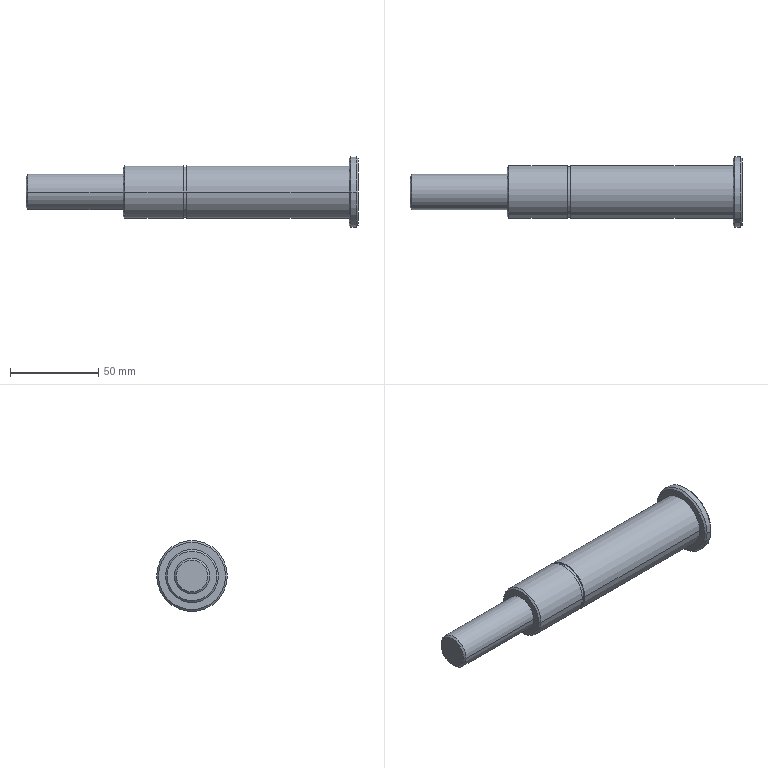Part | SolidWorks | features BaseBody 1 | 1 solid | 24 faces | box 188 x 40 x 40 mm | volume 113711 mm3 | cylinder 10 | cone 8 | plane 6 | commonest cylinder face diameters 30 x4 20 x2 28.6 x2 40 x2
STEP:
#1=CARTESIAN_POINT('',(89.,-19.,0.));
#2=VERTEX_POINT('',#1);
#3=CARTESIAN_POINT('',(89.,19.,0.));
#4=VERTEX_POINT('',#3);
#5=CARTESIAN_POINT('',(89.,0.,0.));
#6=DIRECTION('',(-1.,0.,0.));
#7=DIRECTION('',(0.,1.,0.));
#8=AXIS2_PLACEMENT_3D('',#5,#6,#7);
#9=CIRCLE('',#8,19.);
#10=EDGE_CURVE('',#2,#4,#9,.T.);
#11=ORIENTED_EDGE('',*,*,#10,.F.);
#12=CARTESIAN_POINT('',(90.,-20.,0.));
#13=VERTEX_POINT('',#12);
#14=CARTESIAN_POINT('',(89.,-19.,0.));
#15=DIRECTION('',(0.7071,-0.7071,0.));
#16=VECTOR('',#15,1000.);
#17=LINE('',#14,#16);
#18=EDGE_CURVE('',#2,#13,#17,.T.);
#19=ORIENTED_EDGE('',*,*,#18,.T.);
#20=CARTESIAN_POINT('',(90.,20.,0.));
#21=VERTEX_POINT('',#20);
#22=CARTESIAN_POINT('',(90.,0.,0.));
#23=DIRECTION('',(1.,0.,0.));
#24=DIRECTION('',(0.,1.,0.));
#25=AXIS2_PLACEMENT_3D('',#22,#23,#24);
#26=CIRCLE('',#25,20.);
#27=EDGE_CURVE('',#21,#13,#26,.T.);
#28=ORIENTED_EDGE('',*,*,#27,.F.);
#29=CARTESIAN_POINT('',(89.,19.,0.));
#30=DIRECTION('',(0.7071,0.7071,0.));
#31=VECTOR('',#30,1000.);
#32=LINE('',#29,#31);
#33=EDGE_CURVE('',#4,#21,#32,.T.);
#34=ORIENTED_EDGE('',*,*,#33,.F.);
#35=EDGE_LOOP('',(#11,#19,#28,#34));
#36=FACE_OUTER_BOUND('',#35,.T.);
#37=CARTESIAN_POINT('',(89.,0.,0.));
#38=DIRECTION('',(1.,0.,0.));
#39=DIRECTION('',(0.,1.,0.));
#40=AXIS2_PLACEMENT_3D('',#37,#38,#39);
#41=CONICAL_SURFACE('',#40,19.,0.7854);
#42=ADVANCED_FACE('',(#36),#41,.T.);
#43=CARTESIAN_POINT('',(94.,19.,0.));
#44=VERTEX_POINT('',#43);
#45=CARTESIAN_POINT('',(94.,-19.,0.));
#46=VERTEX_POINT('',#45);
#47=CARTESIAN_POINT('',(94.,0.,0.));
#48=DIRECTION('',(1.,0.,0.));
#49=DIRECTION('',(0.,-1.,0.));
#50=AXIS2_PLACEMENT_3D('',#47,#48,#49);
#51=CIRCLE('',#50,19.);
#52=EDGE_CURVE('',#44,#46,#51,.T.);
#53=ORIENTED_EDGE('',*,*,#52,.F.);
#54=CARTESIAN_POINT('',(93.,20.,0.));
#55=VERTEX_POINT('',#54);
#56=CARTESIAN_POINT('',(93.,20.,0.));
#57=DIRECTION('',(-0.7071,0.7071,0.));
#58=VECTOR('',#57,1000.);
#59=LINE('',#56,#58);
#60=EDGE_CURVE('',#44,#55,#59,.T.);
#61=ORIENTED_EDGE('',*,*,#60,.T.);
#62=CARTESIAN_POINT('',(93.,-20.,0.));
#63=VERTEX_POINT('',#62);
#64=CARTESIAN_POINT('',(93.,0.,0.));
#65=DIRECTION('',(-1.,0.,0.));
#66=DIRECTION('',(0.,-1.,0.));
#67=AXIS2_PLACEMENT_3D('',#64,#65,#66);
#68=CIRCLE('',#67,20.);
#69=EDGE_CURVE('',#63,#55,#68,.T.);
#70=ORIENTED_EDGE('',*,*,#69,.F.);
#71=CARTESIAN_POINT('',(93.,-20.,0.));
#72=DIRECTION('',(-0.7071,-0.7071,0.));
#73=VECTOR('',#72,1000.);
#74=LINE('',#71,#73);
#75=EDGE_CURVE('',#46,#63,#74,.T.);
#76=ORIENTED_EDGE('',*,*,#75,.F.);
#77=EDGE_LOOP('',(#53,#61,#70,#76));
#78=FACE_OUTER_BOUND('',#77,.T.);
#79=CARTESIAN_POINT('',(93.,0.,0.));
#80=DIRECTION('',(-1.,0.,0.));
#81=DIRECTION('',(0.,-1.,0.));
#82=AXIS2_PLACEMENT_3D('',#79,#80,#81);
#83=CONICAL_SURFACE('',#82,20.,0.7854);
#84=ADVANCED_FACE('',(#78),#83,.T.);
#85=CARTESIAN_POINT('',(-94.,-9.,0.));
#86=VERTEX_POINT('',#85);
#87=CARTESIAN_POINT('',(-94.,9.,0.));
#88=VERTEX_POINT('',#87);
#89=CARTESIAN_POINT('',(-94.,0.,0.));
#90=DIRECTION('',(-1.,0.,0.));
#91=DIRECTION('',(0.,-1.,0.));
#92=AXIS2_PLACEMENT_3D('',#89,#90,#91);
#93=CIRCLE('',#92,9.);
#94=EDGE_CURVE('',#86,#88,#93,.T.);
#95=ORIENTED_EDGE('',*,*,#94,.F.);
#96=CARTESIAN_POINT('',(-93.,-10.,0.));
#97=VERTEX_POINT('',#96);
#98=CARTESIAN_POINT('',(-93.,-10.,0.));
#99=DIRECTION('',(0.7071,-0.7071,0.));
#100=VECTOR('',#99,1000.);
#101=LINE('',#98,#100);
#102=EDGE_CURVE('',#86,#97,#101,.T.);
#103=ORIENTED_EDGE('',*,*,#102,.T.);
#104=CARTESIAN_POINT('',(-93.,10.,0.));
#105=VERTEX_POINT('',#104);
#106=CARTESIAN_POINT('',(-93.,0.,0.));
#107=DIRECTION('',(-1.,0.,0.));
#108=DIRECTION('',(0.,-1.,0.));
#109=AXIS2_PLACEMENT_3D('',#106,#107,#108);
#110=CIRCLE('',#109,10.);
#111=EDGE_CURVE('',#97,#105,#110,.T.);
#112=ORIENTED_EDGE('',*,*,#111,.T.);
#113=CARTESIAN_POINT('',(-93.,10.,0.));
#114=DIRECTION('',(0.7071,0.7071,0.));
#115=VECTOR('',#114,1000.);
#116=LINE('',#113,#115);
#117=EDGE_CURVE('',#88,#105,#116,.T.);
#118=ORIENTED_EDGE('',*,*,#117,.F.);
#119=EDGE_LOOP('',(#95,#103,#112,#118));
#120=FACE_OUTER_BOUND('',#119,.T.);
#121=CARTESIAN_POINT('',(-93.,0.,0.));
#122=DIRECTION('',(1.,0.,0.));
#123=DIRECTION('',(0.,1.,0.));
#124=AXIS2_PLACEMENT_3D('',#121,#122,#123);
#125=CONICAL_SURFACE('',#124,10.,0.7854);
#126=ADVANCED_FACE('',(#120),#125,.T.);
#127=CARTESIAN_POINT('',(-39.,-10.,0.));
#128=VERTEX_POINT('',#127);
#129=CARTESIAN_POINT('',(-39.,10.,0.));
#130=VERTEX_POINT('',#129);
#131=CARTESIAN_POINT('',(-39.,0.,0.));
#132=DIRECTION('',(-1.,0.,0.));
#133=DIRECTION('',(0.,-1.,0.));
#134=AXIS2_PLACEMENT_3D('',#131,#132,#133);
#135=CIRCLE('',#134,10.);
#136=EDGE_CURVE('',#128,#130,#135,.T.);
#137=ORIENTED_EDGE('',*,*,#136,.T.);
#138=CARTESIAN_POINT('',(-94.,10.,0.));
#139=DIRECTION('',(-1.,0.,0.));
#140=VECTOR('',#139,1000.);
#141=LINE('',#138,#140);
#142=EDGE_CURVE('',#130,#105,#141,.T.);
#143=ORIENTED_EDGE('',*,*,#142,.T.);
#144=ORIENTED_EDGE('',*,*,#111,.F.);
#145=CARTESIAN_POINT('',(-94.,-10.,0.));
#146=DIRECTION('',(-1.,0.,0.));
#147=VECTOR('',#146,1000.);
#148=LINE('',#145,#147);
#149=EDGE_CURVE('',#128,#97,#148,.T.);
#150=ORIENTED_EDGE('',*,*,#149,.F.);
#151=EDGE_LOOP('',(#137,#143,#144,#150));
#152=FACE_OUTER_BOUND('',#151,.T.);
#153=CARTESIAN_POINT('',(-94.,0.,0.));
#154=DIRECTION('',(-1.,0.,0.));
#155=DIRECTION('',(0.,-1.,0.));
#156=AXIS2_PLACEMENT_3D('',#153,#154,#155);
#157=CYLINDRICAL_SURFACE('',#156,10.);
#158=ADVANCED_FACE('',(#152),#157,.T.);
#159=CARTESIAN_POINT('',(-39.,-14.,0.));
#160=VERTEX_POINT('',#159);
#161=CARTESIAN_POINT('',(-39.,14.,0.));
#162=VERTEX_POINT('',#161);
#163=CARTESIAN_POINT('',(-39.,0.,0.));
#164=DIRECTION('',(-1.,0.,0.));
#165=DIRECTION('',(0.,-1.,0.));
#166=AXIS2_PLACEMENT_3D('',#163,#164,#165);
#167=CIRCLE('',#166,14.);
#168=EDGE_CURVE('',#160,#162,#167,.T.);
#169=ORIENTED_EDGE('',*,*,#168,.F.);
#170=CARTESIAN_POINT('',(-38.,-15.,0.));
#171=VERTEX_POINT('',#170);
#172=CARTESIAN_POINT('',(-38.,-15.,0.));
#173=DIRECTION('',(0.7071,-0.7071,0.));
#174=VECTOR('',#173,1000.);
#175=LINE('',#172,#174);
#176=EDGE_CURVE('',#160,#171,#175,.T.);
#177=ORIENTED_EDGE('',*,*,#176,.T.);
#178=CARTESIAN_POINT('',(-38.,15.,0.));
#179=VERTEX_POINT('',#178);
#180=CARTESIAN_POINT('',(-38.,0.,0.));
#181=DIRECTION('',(-1.,0.,0.));
#182=DIRECTION('',(0.,-1.,0.));
#183=AXIS2_PLACEMENT_3D('',#180,#181,#182);
#184=CIRCLE('',#183,15.);
#185=EDGE_CURVE('',#171,#179,#184,.T.);
#186=ORIENTED_EDGE('',*,*,#185,.T.);
#187=CARTESIAN_POINT('',(-38.,15.,0.));
#188=DIRECTION('',(0.7071,0.7071,0.));
#189=VECTOR('',#188,1000.);
#190=LINE('',#187,#189);
#191=EDGE_CURVE('',#162,#179,#190,.T.);
#192=ORIENTED_EDGE('',*,*,#191,.F.);
#193=EDGE_LOOP('',(#169,#177,#186,#192));
#194=FACE_OUTER_BOUND('',#193,.T.);
#195=CARTESIAN_POINT('',(-38.,0.,0.));
#196=DIRECTION('',(1.,0.,0.));
#197=DIRECTION('',(0.,1.,0.));
#198=AXIS2_PLACEMENT_3D('',#195,#196,#197);
#199=CONICAL_SURFACE('',#198,15.,0.7854);
#200=ADVANCED_FACE('',(#194),#199,.T.);
#201=CARTESIAN_POINT('',(-5.,-15.,0.));
#202=VERTEX_POINT('',#201);
#203=CARTESIAN_POINT('',(-5.,15.,0.));
#204=VERTEX_POINT('',#203);
#205=CARTESIAN_POINT('',(-5.,0.,0.));
#206=DIRECTION('',(-1.,0.,0.));
#207=DIRECTION('',(0.,-1.,0.));
#208=AXIS2_PLACEMENT_3D('',#205,#206,#207);
#209=CIRCLE('',#208,15.);
#210=EDGE_CURVE('',#202,#204,#209,.T.);
#211=ORIENTED_EDGE('',*,*,#210,.T.);
#212=CARTESIAN_POINT('',(-94.,15.,0.));
#213=DIRECTION('',(-1.,0.,0.));
#214=VECTOR('',#213,1000.);
#215=LINE('',#212,#214);
#216=EDGE_CURVE('',#204,#179,#215,.T.);
#217=ORIENTED_EDGE('',*,*,#216,.T.);
#218=ORIENTED_EDGE('',*,*,#185,.F.);
#219=CARTESIAN_POINT('',(-94.,-15.,0.));
#220=DIRECTION('',(-1.,0.,0.));
#221=VECTOR('',#220,1000.);
#222=LINE('',#219,#221);
#223=EDGE_CURVE('',#202,#171,#222,.T.);
#224=ORIENTED_EDGE('',*,*,#223,.F.);
#225=EDGE_LOOP('',(#211,#217,#218,#224));
#226=FACE_OUTER_BOUND('',#225,.T.);
#227=CARTESIAN_POINT('',(-94.,0.,0.));
#228=DIRECTION('',(-1.,0.,0.));
#229=DIRECTION('',(0.,-1.,0.));
#230=AXIS2_PLACEMENT_3D('',#227,#228,#229);
#231=CYLINDRICAL_SURFACE('',#230,15.);
#232=ADVANCED_FACE('',(#226),#231,.T.);
#233=CARTESIAN_POINT('',(-3.,-14.3,0.));
#234=VERTEX_POINT('',#233);
#235=CARTESIAN_POINT('',(-3.,14.3,0.));
#236=VERTEX_POINT('',#235);
#237=CARTESIAN_POINT('',(-3.,0.,0.));
#238=DIRECTION('',(-1.,0.,0.));
#239=DIRECTION('',(0.,-1.,0.));
#240=AXIS2_PLACEMENT_3D('',#237,#238,#239);
#241=CIRCLE('',#240,14.3);
#242=EDGE_CURVE('',#234,#236,#241,.T.);
#243=ORIENTED_EDGE('',*,*,#242,.T.);
#244=CARTESIAN_POINT('',(-5.,14.3,0.));
#245=VERTEX_POINT('',#244);
#246=CARTESIAN_POINT('',(-94.,14.3,0.));
#247=DIRECTION('',(-1.,0.,0.));
#248=VECTOR('',#247,1000.);
#249=LINE('',#246,#248);
#250=EDGE_CURVE('',#236,#245,#249,.T.);
#251=ORIENTED_EDGE('',*,*,#250,.T.);
#252=CARTESIAN_POINT('',(-5.,-14.3,0.));
#253=VERTEX_POINT('',#252);
#254=CARTESIAN_POINT('',(-5.,0.,0.));
#255=DIRECTION('',(-1.,0.,0.));
#256=DIRECTION('',(0.,-1.,0.));
#257=AXIS2_PLACEMENT_3D('',#254,#255,#256);
#258=CIRCLE('',#257,14.3);
#259=EDGE_CURVE('',#253,#245,#258,.T.);
#260=ORIENTED_EDGE('',*,*,#259,.F.);
#261=CARTESIAN_POINT('',(-94.,-14.3,0.));
#262=DIRECTION('',(-1.,0.,0.));
#263=VECTOR('',#262,1000.);
#264=LINE('',#261,#263);
#265=EDGE_CURVE('',#234,#253,#264,.T.);
#266=ORIENTED_EDGE('',*,*,#265,.F.);
#267=EDGE_LOOP('',(#243,#251,#260,#266));
#268=FACE_OUTER_BOUND('',#267,.T.);
#269=CARTESIAN_POINT('',(-94.,0.,0.));
#270=DIRECTION('',(-1.,0.,0.));
#271=DIRECTION('',(0.,-1.,0.));
#272=AXIS2_PLACEMENT_3D('',#269,#270,#271);
#273=CYLINDRICAL_SURFACE('',#272,14.3);
#274=ADVANCED_FACE('',(#268),#273,.T.);
#275=CARTESIAN_POINT('',(89.,-15.,0.));
#276=VERTEX_POINT('',#275);
#277=CARTESIAN_POINT('',(89.,15.,0.));
#278=VERTEX_POINT('',#277);
#279=CARTESIAN_POINT('',(89.,0.,0.));
#280=DIRECTION('',(-1.,0.,0.));
#281=DIRECTION('',(0.,-1.,0.));
#282=AXIS2_PLACEMENT_3D('',#279,#280,#281);
#283=CIRCLE('',#282,15.);
#284=EDGE_CURVE('',#276,#278,#283,.T.);
#285=ORIENTED_EDGE('',*,*,#284,.T.);
#286=CARTESIAN_POINT('',(-3.,15.,0.));
#287=VERTEX_POINT('',#286);
#288=CARTESIAN_POINT('',(-94.,15.,0.));
#289=DIRECTION('',(-1.,0.,0.));
#290=VECTOR('',#289,1000.);
#291=LINE('',#288,#290);
#292=EDGE_CURVE('',#278,#287,#291,.T.);
#293=ORIENTED_EDGE('',*,*,#292,.T.);
#294=CARTESIAN_POINT('',(-3.,-15.,0.));
#295=VERTEX_POINT('',#294);
#296=CARTESIAN_POINT('',(-3.,0.,0.));
#297=DIRECTION('',(-1.,0.,0.));
#298=DIRECTION('',(0.,-1.,0.));
#299=AXIS2_PLACEMENT_3D('',#296,#297,#298);
#300=CIRCLE('',#299,15.);
#301=EDGE_CURVE('',#295,#287,#300,.T.);
#302=ORIENTED_EDGE('',*,*,#301,.F.);
#303=CARTESIAN_POINT('',(-94.,-15.,0.));
#304=DIRECTION('',(-1.,0.,0.));
#305=VECTOR('',#304,1000.);
#306=LINE('',#303,#305);
#307=EDGE_CURVE('',#276,#295,#306,.T.);
#308=ORIENTED_EDGE('',*,*,#307,.F.);
#309=EDGE_LOOP('',(#285,#293,#302,#308));
#310=FACE_OUTER_BOUND('',#309,.T.);
#311=CARTESIAN_POINT('',(-94.,0.,0.));
#312=DIRECTION('',(-1.,0.,0.));
#313=DIRECTION('',(0.,-1.,0.));
#314=AXIS2_PLACEMENT_3D('',#311,#312,#313);
#315=CYLINDRICAL_SURFACE('',#314,15.);
#316=ADVANCED_FACE('',(#310),#315,.T.);
#317=ORIENTED_EDGE('',*,*,#69,.T.);
#318=CARTESIAN_POINT('',(-94.,20.,0.));
#319=DIRECTION('',(-1.,0.,0.));
#320=VECTOR('',#319,1000.);
#321=LINE('',#318,#320);
#322=EDGE_CURVE('',#55,#21,#321,.T.);
#323=ORIENTED_EDGE('',*,*,#322,.T.);
#324=ORIENTED_EDGE('',*,*,#27,.T.);
#325=CARTESIAN_POINT('',(-94.,-20.,0.));
#326=DIRECTION('',(-1.,0.,0.));
#327=VECTOR('',#326,1000.);
#328=LINE('',#325,#327);
#329=EDGE_CURVE('',#63,#13,#328,.T.);
#330=ORIENTED_EDGE('',*,*,#329,.F.);
#331=EDGE_LOOP('',(#317,#323,#324,#330));
#332=FACE_OUTER_BOUND('',#331,.T.);
#333=CARTESIAN_POINT('',(-94.,0.,0.));
#334=DIRECTION('',(-1.,0.,0.));
#335=DIRECTION('',(0.,-1.,0.));
#336=AXIS2_PLACEMENT_3D('',#333,#334,#335);
#337=CYLINDRICAL_SURFACE('',#336,20.);
#338=ADVANCED_FACE('',(#332),#337,.T.);
#339=CARTESIAN_POINT('',(94.,0.,0.));
#340=DIRECTION('',(1.,0.,0.));
#341=DIRECTION('',(0.,-1.,0.));
#342=AXIS2_PLACEMENT_3D('',#339,#340,#341);
#343=CIRCLE('',#342,19.);
#344=EDGE_CURVE('',#46,#44,#343,.T.);
#345=ORIENTED_EDGE('',*,*,#344,.T.);
#346=ORIENTED_EDGE('',*,*,#52,.T.);
#347=EDGE_LOOP('',(#345,#346));
#348=FACE_OUTER_BOUND('',#347,.T.);
#349=CARTESIAN_POINT('',(94.,0.,0.));
#350=DIRECTION('',(-1.,0.,0.));
#351=DIRECTION('',(0.,-1.,0.));
#352=AXIS2_PLACEMENT_3D('',#349,#350,#351);
#353=PLANE('',#352);
#354=ADVANCED_FACE('',(#348),#353,.F.);
#355=ORIENTED_EDGE('',*,*,#322,.F.);
#356=CARTESIAN_POINT('',(93.,0.,0.));
#357=DIRECTION('',(-1.,0.,0.));
#358=DIRECTION('',(0.,-1.,0.));
#359=AXIS2_PLACEMENT_3D('',#356,#357,#358);
#360=CIRCLE('',#359,20.);
#361=EDGE_CURVE('',#55,#63,#360,.T.);
#362=ORIENTED_EDGE('',*,*,#361,.T.);
#363=ORIENTED_EDGE('',*,*,#329,.T.);
#364=CARTESIAN_POINT('',(90.,0.,0.));
#365=DIRECTION('',(1.,0.,0.));
#366=DIRECTION('',(0.,1.,0.));
#367=AXIS2_PLACEMENT_3D('',#364,#365,#366);
#368=CIRCLE('',#367,20.);
#369=EDGE_CURVE('',#13,#21,#368,.T.);
#370=ORIENTED_EDGE('',*,*,#369,.T.);
#371=EDGE_LOOP('',(#355,#362,#363,#370));
#372=FACE_OUTER_BOUND('',#371,.T.);
#373=CARTESIAN_POINT('',(-94.,0.,0.));
#374=DIRECTION('',(-1.,0.,0.));
#375=DIRECTION('',(0.,-1.,0.));
#376=AXIS2_PLACEMENT_3D('',#373,#374,#375);
#377=CYLINDRICAL_SURFACE('',#376,20.);
#378=ADVANCED_FACE('',(#372),#377,.T.);
#379=CARTESIAN_POINT('',(89.,0.,0.));
#380=DIRECTION('',(-1.,0.,0.));
#381=DIRECTION('',(0.,1.,0.));
#382=AXIS2_PLACEMENT_3D('',#379,#380,#381);
#383=CIRCLE('',#382,19.);
#384=EDGE_CURVE('',#4,#2,#383,.T.);
#385=ORIENTED_EDGE('',*,*,#384,.T.);
#386=ORIENTED_EDGE('',*,*,#10,.T.);
#387=EDGE_LOOP('',(#385,#386));
#388=FACE_OUTER_BOUND('',#387,.T.);
#389=ORIENTED_EDGE('',*,*,#284,.F.);
#390=CARTESIAN_POINT('',(89.,0.,0.));
#391=DIRECTION('',(-1.,0.,0.));
#392=DIRECTION('',(0.,-1.,0.));
#393=AXIS2_PLACEMENT_3D('',#390,#391,#392);
#394=CIRCLE('',#393,15.);
#395=EDGE_CURVE('',#278,#276,#394,.T.);
#396=ORIENTED_EDGE('',*,*,#395,.F.);
#397=EDGE_LOOP('',(#389,#396));
#398=FACE_BOUND('',#397,.T.);
#399=CARTESIAN_POINT('',(89.,20.,0.));
#400=DIRECTION('',(1.,0.,0.));
#401=DIRECTION('',(0.,1.,0.));
#402=AXIS2_PLACEMENT_3D('',#399,#400,#401);
#403=PLANE('',#402);
#404=ADVANCED_FACE('',(#388,#398),#403,.F.);
#405=ORIENTED_EDGE('',*,*,#292,.F.);
#406=ORIENTED_EDGE('',*,*,#395,.T.);
#407=ORIENTED_EDGE('',*,*,#307,.T.);
#408=CARTESIAN_POINT('',(-3.,0.,0.));
#409=DIRECTION('',(-1.,0.,0.));
#410=DIRECTION('',(0.,-1.,0.));
#411=AXIS2_PLACEMENT_3D('',#408,#409,#410);
#412=CIRCLE('',#411,15.);
#413=EDGE_CURVE('',#287,#295,#412,.T.);
#414=ORIENTED_EDGE('',*,*,#413,.F.);
#415=EDGE_LOOP('',(#405,#406,#407,#414));
#416=FACE_OUTER_BOUND('',#415,.T.);
#417=CARTESIAN_POINT('',(-94.,0.,0.));
#418=DIRECTION('',(-1.,0.,0.));
#419=DIRECTION('',(0.,-1.,0.));
#420=AXIS2_PLACEMENT_3D('',#417,#418,#419);
#421=CYLINDRICAL_SURFACE('',#420,15.);
#422=ADVANCED_FACE('',(#416),#421,.T.);
#423=ORIENTED_EDGE('',*,*,#242,.F.);
#424=CARTESIAN_POINT('',(-3.,0.,0.));
#425=DIRECTION('',(-1.,0.,0.));
#426=DIRECTION('',(0.,-1.,0.));
#427=AXIS2_PLACEMENT_3D('',#424,#425,#426);
#428=CIRCLE('',#427,14.3);
#429=EDGE_CURVE('',#236,#234,#428,.T.);
#430=ORIENTED_EDGE('',*,*,#429,.F.);
#431=EDGE_LOOP('',(#423,#430));
#432=FACE_BOUND('',#431,.T.);
#433=ORIENTED_EDGE('',*,*,#301,.T.);
#434=ORIENTED_EDGE('',*,*,#413,.T.);
#435=EDGE_LOOP('',(#433,#434));
#436=FACE_OUTER_BOUND('',#435,.T.);
#437=CARTESIAN_POINT('',(-3.,15.,0.));
#438=DIRECTION('',(1.,0.,0.));
#439=DIRECTION('',(0.,1.,0.));
#440=AXIS2_PLACEMENT_3D('',#437,#438,#439);
#441=PLANE('',#440);
#442=ADVANCED_FACE('',(#432,#436),#441,.F.);
#443=ORIENTED_EDGE('',*,*,#250,.F.);
#444=ORIENTED_EDGE('',*,*,#429,.T.);
#445=ORIENTED_EDGE('',*,*,#265,.T.);
#446=CARTESIAN_POINT('',(-5.,0.,0.));
#447=DIRECTION('',(-1.,0.,0.));
#448=DIRECTION('',(0.,-1.,0.));
#449=AXIS2_PLACEMENT_3D('',#446,#447,#448);
#450=CIRCLE('',#449,14.3);
#451=EDGE_CURVE('',#245,#253,#450,.T.);
#452=ORIENTED_EDGE('',*,*,#451,.F.);
#453=EDGE_LOOP('',(#443,#444,#445,#452));
#454=FACE_OUTER_BOUND('',#453,.T.);
#455=CARTESIAN_POINT('',(-94.,0.,0.));
#456=DIRECTION('',(-1.,0.,0.));
#457=DIRECTION('',(0.,-1.,0.));
#458=AXIS2_PLACEMENT_3D('',#455,#456,#457);
#459=CYLINDRICAL_SURFACE('',#458,14.3);
#460=ADVANCED_FACE('',(#454),#459,.T.);
#461=ORIENTED_EDGE('',*,*,#210,.F.);
#462=CARTESIAN_POINT('',(-5.,0.,0.));
#463=DIRECTION('',(-1.,0.,0.));
#464=DIRECTION('',(0.,-1.,0.));
#465=AXIS2_PLACEMENT_3D('',#462,#463,#464);
#466=CIRCLE('',#465,15.);
#467=EDGE_CURVE('',#204,#202,#466,.T.);
#468=ORIENTED_EDGE('',*,*,#467,.F.);
#469=EDGE_LOOP('',(#461,#468));
#470=FACE_OUTER_BOUND('',#469,.T.);
#471=ORIENTED_EDGE('',*,*,#259,.T.);
#472=ORIENTED_EDGE('',*,*,#451,.T.);
#473=EDGE_LOOP('',(#471,#472));
#474=FACE_BOUND('',#473,.T.);
#475=CARTESIAN_POINT('',(-5.,15.,0.));
#476=DIRECTION('',(-1.,0.,0.));
#477=DIRECTION('',(0.,-1.,0.));
#478=AXIS2_PLACEMENT_3D('',#475,#476,#477);
#479=PLANE('',#478);
#480=ADVANCED_FACE('',(#470,#474),#479,.F.);
#481=ORIENTED_EDGE('',*,*,#216,.F.);
#482=ORIENTED_EDGE('',*,*,#467,.T.);
#483=ORIENTED_EDGE('',*,*,#223,.T.);
#484=CARTESIAN_POINT('',(-38.,0.,0.));
#485=DIRECTION('',(-1.,0.,0.));
#486=DIRECTION('',(0.,-1.,0.));
#487=AXIS2_PLACEMENT_3D('',#484,#485,#486);
#488=CIRCLE('',#487,15.);
#489=EDGE_CURVE('',#179,#171,#488,.T.);
#490=ORIENTED_EDGE('',*,*,#489,.F.);
#491=EDGE_LOOP('',(#481,#482,#483,#490));
#492=FACE_OUTER_BOUND('',#491,.T.);
#493=CARTESIAN_POINT('',(-94.,0.,0.));
#494=DIRECTION('',(-1.,0.,0.));
#495=DIRECTION('',(0.,-1.,0.));
#496=AXIS2_PLACEMENT_3D('',#493,#494,#495);
#497=CYLINDRICAL_SURFACE('',#496,15.);
#498=ADVANCED_FACE('',(#492),#497,.T.);
#499=ORIENTED_EDGE('',*,*,#176,.F.);
#500=CARTESIAN_POINT('',(-39.,0.,0.));
#501=DIRECTION('',(-1.,0.,0.));
#502=DIRECTION('',(0.,-1.,0.));
#503=AXIS2_PLACEMENT_3D('',#500,#501,#502);
#504=CIRCLE('',#503,14.);
#505=EDGE_CURVE('',#162,#160,#504,.T.);
#506=ORIENTED_EDGE('',*,*,#505,.F.);
#507=ORIENTED_EDGE('',*,*,#191,.T.);
#508=ORIENTED_EDGE('',*,*,#489,.T.);
#509=EDGE_LOOP('',(#499,#506,#507,#508));
#510=FACE_OUTER_BOUND('',#509,.T.);
#511=CARTESIAN_POINT('',(-38.,0.,0.));
#512=DIRECTION('',(1.,0.,0.));
#513=DIRECTION('',(0.,1.,0.));
#514=AXIS2_PLACEMENT_3D('',#511,#512,#513);
#515=CONICAL_SURFACE('',#514,15.,0.7854);
#516=ADVANCED_FACE('',(#510),#515,.T.);
#517=ORIENTED_EDGE('',*,*,#136,.F.);
#518=CARTESIAN_POINT('',(-39.,0.,0.));
#519=DIRECTION('',(-1.,0.,0.));
#520=DIRECTION('',(0.,-1.,0.));
#521=AXIS2_PLACEMENT_3D('',#518,#519,#520);
#522=CIRCLE('',#521,10.);
#523=EDGE_CURVE('',#130,#128,#522,.T.);
#524=ORIENTED_EDGE('',*,*,#523,.F.);
#525=EDGE_LOOP('',(#517,#524));
#526=FACE_BOUND('',#525,.T.);
#527=ORIENTED_EDGE('',*,*,#505,.T.);
#528=ORIENTED_EDGE('',*,*,#168,.T.);
#529=EDGE_LOOP('',(#527,#528));
#530=FACE_OUTER_BOUND('',#529,.T.);
#531=CARTESIAN_POINT('',(-39.,10.,0.));
#532=DIRECTION('',(1.,0.,0.));
#533=DIRECTION('',(0.,1.,0.));
#534=AXIS2_PLACEMENT_3D('',#531,#532,#533);
#535=PLANE('',#534);
#536=ADVANCED_FACE('',(#526,#530),#535,.F.);
#537=ORIENTED_EDGE('',*,*,#142,.F.);
#538=ORIENTED_EDGE('',*,*,#523,.T.);
#539=ORIENTED_EDGE('',*,*,#149,.T.);
#540=CARTESIAN_POINT('',(-93.,0.,0.));
#541=DIRECTION('',(-1.,0.,0.));
#542=DIRECTION('',(0.,-1.,0.));
#543=AXIS2_PLACEMENT_3D('',#540,#541,#542);
#544=CIRCLE('',#543,10.);
#545=EDGE_CURVE('',#105,#97,#544,.T.);
#546=ORIENTED_EDGE('',*,*,#545,.F.);
#547=EDGE_LOOP('',(#537,#538,#539,#546));
#548=FACE_OUTER_BOUND('',#547,.T.);
#549=CARTESIAN_POINT('',(-94.,0.,0.));
#550=DIRECTION('',(-1.,0.,0.));
#551=DIRECTION('',(0.,-1.,0.));
#552=AXIS2_PLACEMENT_3D('',#549,#550,#551);
#553=CYLINDRICAL_SURFACE('',#552,10.);
#554=ADVANCED_FACE('',(#548),#553,.T.);
#555=ORIENTED_EDGE('',*,*,#102,.F.);
#556=CARTESIAN_POINT('',(-94.,0.,0.));
#557=DIRECTION('',(-1.,0.,0.));
#558=DIRECTION('',(0.,-1.,0.));
#559=AXIS2_PLACEMENT_3D('',#556,#557,#558);
#560=CIRCLE('',#559,9.);
#561=EDGE_CURVE('',#88,#86,#560,.T.);
#562=ORIENTED_EDGE('',*,*,#561,.F.);
#563=ORIENTED_EDGE('',*,*,#117,.T.);
#564=ORIENTED_EDGE('',*,*,#545,.T.);
#565=EDGE_LOOP('',(#555,#562,#563,#564));
#566=FACE_OUTER_BOUND('',#565,.T.);
#567=CARTESIAN_POINT('',(-93.,0.,0.));
#568=DIRECTION('',(1.,0.,0.));
#569=DIRECTION('',(0.,1.,0.));
#570=AXIS2_PLACEMENT_3D('',#567,#568,#569);
#571=CONICAL_SURFACE('',#570,10.,0.7854);
#572=ADVANCED_FACE('',(#566),#571,.T.);
#573=ORIENTED_EDGE('',*,*,#561,.T.);
#574=ORIENTED_EDGE('',*,*,#94,.T.);
#575=EDGE_LOOP('',(#573,#574));
#576=FACE_OUTER_BOUND('',#575,.T.);
#577=CARTESIAN_POINT('',(-94.,9.,0.));
#578=DIRECTION('',(1.,0.,0.));
#579=DIRECTION('',(0.,1.,0.));
#580=AXIS2_PLACEMENT_3D('',#577,#578,#579);
#581=PLANE('',#580);
#582=ADVANCED_FACE('',(#576),#581,.F.);
#583=ORIENTED_EDGE('',*,*,#60,.F.);
#584=ORIENTED_EDGE('',*,*,#344,.F.);
#585=ORIENTED_EDGE('',*,*,#75,.T.);
#586=ORIENTED_EDGE('',*,*,#361,.F.);
#587=EDGE_LOOP('',(#583,#584,#585,#586));
#588=FACE_OUTER_BOUND('',#587,.T.);
#589=CARTESIAN_POINT('',(93.,0.,0.));
#590=DIRECTION('',(-1.,0.,0.));
#591=DIRECTION('',(0.,-1.,0.));
#592=AXIS2_PLACEMENT_3D('',#589,#590,#591);
#593=CONICAL_SURFACE('',#592,20.,0.7854);
#594=ADVANCED_FACE('',(#588),#593,.T.);
#595=ORIENTED_EDGE('',*,*,#18,.F.);
#596=ORIENTED_EDGE('',*,*,#384,.F.);
#597=ORIENTED_EDGE('',*,*,#33,.T.);
#598=ORIENTED_EDGE('',*,*,#369,.F.);
#599=EDGE_LOOP('',(#595,#596,#597,#598));
#600=FACE_OUTER_BOUND('',#599,.T.);
#601=CARTESIAN_POINT('',(89.,0.,0.));
#602=DIRECTION('',(1.,0.,0.));
#603=DIRECTION('',(0.,1.,0.));
#604=AXIS2_PLACEMENT_3D('',#601,#602,#603);
#605=CONICAL_SURFACE('',#604,19.,0.7854);
#606=ADVANCED_FACE('',(#600),#605,.T.);
#607=CLOSED_SHELL('',(#42,#84,#126,#158,#200,#232,#274,#316,#338,#354,#378,#404,#422,#442,#460,#480,#498,#516,#536,#554,#572,#582,#594,#606));
#608=MANIFOLD_SOLID_BREP('',#607);
#609=CARTESIAN_POINT('',(0.,0.,0.));
#610=DIRECTION('',(0.,0.,1.));
#611=DIRECTION('',(1.,0.,0.));
#612=AXIS2_PLACEMENT_3D('',#609,#610,#611);
#613=(LENGTH_UNIT()NAMED_UNIT(*)SI_UNIT(.MILLI.,.METRE.));
#614=UNCERTAINTY_MEASURE_WITH_UNIT(LENGTH_MEASURE(0.00001),#613,'','');
#615=(NAMED_UNIT(*)PLANE_ANGLE_UNIT()SI_UNIT($,.RADIAN.));
#616=(NAMED_UNIT(*)SI_UNIT($,.STERADIAN.)SOLID_ANGLE_UNIT());
#617=(GEOMETRIC_REPRESENTATION_CONTEXT(3)GLOBAL_UNCERTAINTY_ASSIGNED_CONTEXT((#614))GLOBAL_UNIT_ASSIGNED_CONTEXT((#613,#615,#616))REPRESENTATION_CONTEXT('',''));
#618=ADVANCED_BREP_SHAPE_REPRESENTATION('',(#608,#612),#617);